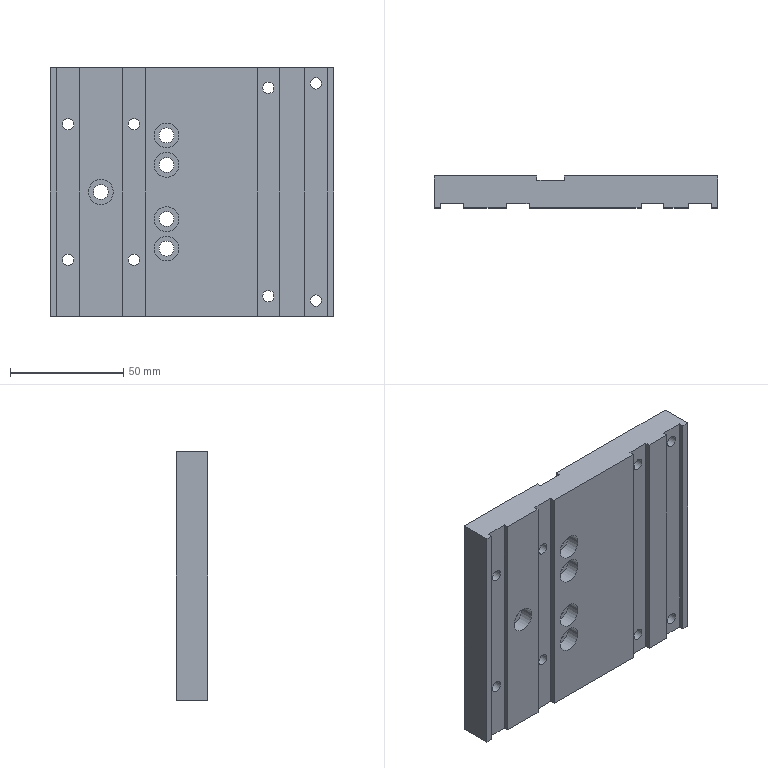Part | 1 solid | 49 faces | box 125.5 x 14 x 110 mm | volume 175999 mm3 | plane 31 | cylinder 18 | commonest cylinder face diameters 5 x8 6.6 x5 11 x5
STEP:
#1=CARTESIAN_POINT('',(93.5,0.,-78.5));
#2=VERTEX_POINT('',#1);
#3=CARTESIAN_POINT('',(93.5,0.,-76.));
#4=DIRECTION('',(0.,1.,0.));
#5=DIRECTION('',(0.,0.,-1.));
#6=AXIS2_PLACEMENT_3D('',#3,#4,#5);
#7=CIRCLE('',#6,2.5);
#8=EDGE_CURVE('',#2,#2,#7,.T.);
#9=ORIENTED_EDGE('',*,*,#8,.F.);
#10=EDGE_LOOP('',(#9));
#11=FACE_BOUND('',#10,.T.);
#12=CARTESIAN_POINT('',(93.5,12.,-78.5));
#13=VERTEX_POINT('',#12);
#14=CARTESIAN_POINT('',(93.5,12.,-76.));
#15=DIRECTION('',(0.,1.,0.));
#16=DIRECTION('',(0.,0.,-1.));
#17=AXIS2_PLACEMENT_3D('',#14,#15,#16);
#18=CIRCLE('',#17,2.5);
#19=EDGE_CURVE('',#13,#13,#18,.T.);
#20=ORIENTED_EDGE('',*,*,#19,.T.);
#21=EDGE_LOOP('',(#20));
#22=FACE_BOUND('',#21,.T.);
#23=CARTESIAN_POINT('',(93.5,12.001,-76.));
#24=DIRECTION('',(0.,-1.,0.));
#25=DIRECTION('',(0.,0.,1.));
#26=AXIS2_PLACEMENT_3D('',#23,#24,#25);
#27=CYLINDRICAL_SURFACE('',#26,2.5);
#28=ADVANCED_FACE('',(#11,#22),#27,.F.);
#29=CARTESIAN_POINT('',(93.5,0.,13.5));
#30=VERTEX_POINT('',#29);
#31=CARTESIAN_POINT('',(93.5,0.,16.));
#32=DIRECTION('',(0.,1.,0.));
#33=DIRECTION('',(0.,0.,-1.));
#34=AXIS2_PLACEMENT_3D('',#31,#32,#33);
#35=CIRCLE('',#34,2.5);
#36=EDGE_CURVE('',#30,#30,#35,.T.);
#37=ORIENTED_EDGE('',*,*,#36,.F.);
#38=EDGE_LOOP('',(#37));
#39=FACE_BOUND('',#38,.T.);
#40=CARTESIAN_POINT('',(93.5,12.,13.5));
#41=VERTEX_POINT('',#40);
#42=CARTESIAN_POINT('',(93.5,12.,16.));
#43=DIRECTION('',(0.,1.,0.));
#44=DIRECTION('',(0.,0.,-1.));
#45=AXIS2_PLACEMENT_3D('',#42,#43,#44);
#46=CIRCLE('',#45,2.5);
#47=EDGE_CURVE('',#41,#41,#46,.T.);
#48=ORIENTED_EDGE('',*,*,#47,.T.);
#49=EDGE_LOOP('',(#48));
#50=FACE_BOUND('',#49,.T.);
#51=CARTESIAN_POINT('',(93.5,12.001,16.));
#52=DIRECTION('',(0.,-1.,0.));
#53=DIRECTION('',(0.,0.,1.));
#54=AXIS2_PLACEMENT_3D('',#51,#52,#53);
#55=CYLINDRICAL_SURFACE('',#54,2.5);
#56=ADVANCED_FACE('',(#39,#50),#55,.F.);
#57=CARTESIAN_POINT('',(114.5,0.,-80.5));
#58=VERTEX_POINT('',#57);
#59=CARTESIAN_POINT('',(114.5,0.,-78.));
#60=DIRECTION('',(0.,-1.,0.));
#61=DIRECTION('',(0.,0.,-1.));
#62=AXIS2_PLACEMENT_3D('',#59,#60,#61);
#63=CIRCLE('',#62,2.5);
#64=EDGE_CURVE('',#58,#58,#63,.T.);
#65=ORIENTED_EDGE('',*,*,#64,.T.);
#66=EDGE_LOOP('',(#65));
#67=FACE_BOUND('',#66,.T.);
#68=CARTESIAN_POINT('',(114.5,12.,-80.5));
#69=VERTEX_POINT('',#68);
#70=CARTESIAN_POINT('',(114.5,12.,-78.));
#71=DIRECTION('',(0.,1.,0.));
#72=DIRECTION('',(0.,0.,-1.));
#73=AXIS2_PLACEMENT_3D('',#70,#71,#72);
#74=CIRCLE('',#73,2.5);
#75=EDGE_CURVE('',#69,#69,#74,.T.);
#76=ORIENTED_EDGE('',*,*,#75,.T.);
#77=EDGE_LOOP('',(#76));
#78=FACE_BOUND('',#77,.T.);
#79=CARTESIAN_POINT('',(114.5,19.071,-78.));
#80=DIRECTION('',(0.,-1.,0.));
#81=DIRECTION('',(0.,0.,1.));
#82=AXIS2_PLACEMENT_3D('',#79,#80,#81);
#83=CYLINDRICAL_SURFACE('',#82,2.5);
#84=ADVANCED_FACE('',(#67,#78),#83,.F.);
#85=CARTESIAN_POINT('',(114.5,0.,15.5));
#86=VERTEX_POINT('',#85);
#87=CARTESIAN_POINT('',(114.5,0.,18.));
#88=DIRECTION('',(0.,-1.,0.));
#89=DIRECTION('',(0.,0.,-1.));
#90=AXIS2_PLACEMENT_3D('',#87,#88,#89);
#91=CIRCLE('',#90,2.5);
#92=EDGE_CURVE('',#86,#86,#91,.T.);
#93=ORIENTED_EDGE('',*,*,#92,.T.);
#94=EDGE_LOOP('',(#93));
#95=FACE_BOUND('',#94,.T.);
#96=CARTESIAN_POINT('',(114.5,12.,15.5));
#97=VERTEX_POINT('',#96);
#98=CARTESIAN_POINT('',(114.5,12.,18.));
#99=DIRECTION('',(0.,1.,0.));
#100=DIRECTION('',(0.,0.,-1.));
#101=AXIS2_PLACEMENT_3D('',#98,#99,#100);
#102=CIRCLE('',#101,2.5);
#103=EDGE_CURVE('',#97,#97,#102,.T.);
#104=ORIENTED_EDGE('',*,*,#103,.T.);
#105=EDGE_LOOP('',(#104));
#106=FACE_BOUND('',#105,.T.);
#107=CARTESIAN_POINT('',(114.5,19.071,18.));
#108=DIRECTION('',(0.,-1.,0.));
#109=DIRECTION('',(0.,0.,1.));
#110=AXIS2_PLACEMENT_3D('',#107,#108,#109);
#111=CYLINDRICAL_SURFACE('',#110,2.5);
#112=ADVANCED_FACE('',(#95,#106),#111,.F.);
#113=CARTESIAN_POINT('',(34.,0.,-62.5));
#114=VERTEX_POINT('',#113);
#115=CARTESIAN_POINT('',(34.,0.,-60.));
#116=DIRECTION('',(0.,-1.,0.));
#117=DIRECTION('',(0.,0.,-1.));
#118=AXIS2_PLACEMENT_3D('',#115,#116,#117);
#119=CIRCLE('',#118,2.5);
#120=EDGE_CURVE('',#114,#114,#119,.T.);
#121=ORIENTED_EDGE('',*,*,#120,.T.);
#122=EDGE_LOOP('',(#121));
#123=FACE_BOUND('',#122,.T.);
#124=CARTESIAN_POINT('',(34.,12.,-62.5));
#125=VERTEX_POINT('',#124);
#126=CARTESIAN_POINT('',(34.,12.,-60.));
#127=DIRECTION('',(0.,1.,0.));
#128=DIRECTION('',(0.,0.,-1.));
#129=AXIS2_PLACEMENT_3D('',#126,#127,#128);
#130=CIRCLE('',#129,2.5);
#131=EDGE_CURVE('',#125,#125,#130,.T.);
#132=ORIENTED_EDGE('',*,*,#131,.T.);
#133=EDGE_LOOP('',(#132));
#134=FACE_BOUND('',#133,.T.);
#135=CARTESIAN_POINT('',(34.,19.071,-60.));
#136=DIRECTION('',(0.,-1.,0.));
#137=DIRECTION('',(0.,0.,1.));
#138=AXIS2_PLACEMENT_3D('',#135,#136,#137);
#139=CYLINDRICAL_SURFACE('',#138,2.5);
#140=ADVANCED_FACE('',(#123,#134),#139,.F.);
#141=CARTESIAN_POINT('',(34.,0.,-2.5));
#142=VERTEX_POINT('',#141);
#143=CARTESIAN_POINT('',(34.,0.,0.));
#144=DIRECTION('',(0.,-1.,0.));
#145=DIRECTION('',(0.,0.,-1.));
#146=AXIS2_PLACEMENT_3D('',#143,#144,#145);
#147=CIRCLE('',#146,2.5);
#148=EDGE_CURVE('',#142,#142,#147,.T.);
#149=ORIENTED_EDGE('',*,*,#148,.T.);
#150=EDGE_LOOP('',(#149));
#151=FACE_BOUND('',#150,.T.);
#152=CARTESIAN_POINT('',(34.,12.,-2.5));
#153=VERTEX_POINT('',#152);
#154=CARTESIAN_POINT('',(34.,12.,0.));
#155=DIRECTION('',(0.,1.,0.));
#156=DIRECTION('',(0.,0.,-1.));
#157=AXIS2_PLACEMENT_3D('',#154,#155,#156);
#158=CIRCLE('',#157,2.5);
#159=EDGE_CURVE('',#153,#153,#158,.T.);
#160=ORIENTED_EDGE('',*,*,#159,.T.);
#161=EDGE_LOOP('',(#160));
#162=FACE_BOUND('',#161,.T.);
#163=CARTESIAN_POINT('',(34.,19.071,0.));
#164=DIRECTION('',(0.,-1.,0.));
#165=DIRECTION('',(0.,0.,1.));
#166=AXIS2_PLACEMENT_3D('',#163,#164,#165);
#167=CYLINDRICAL_SURFACE('',#166,2.5);
#168=ADVANCED_FACE('',(#151,#162),#167,.F.);
#169=CARTESIAN_POINT('',(5.,0.,-62.5));
#170=VERTEX_POINT('',#169);
#171=CARTESIAN_POINT('',(5.,0.,-60.));
#172=DIRECTION('',(0.,-1.,0.));
#173=DIRECTION('',(0.,0.,-1.));
#174=AXIS2_PLACEMENT_3D('',#171,#172,#173);
#175=CIRCLE('',#174,2.5);
#176=EDGE_CURVE('',#170,#170,#175,.T.);
#177=ORIENTED_EDGE('',*,*,#176,.T.);
#178=EDGE_LOOP('',(#177));
#179=FACE_BOUND('',#178,.T.);
#180=CARTESIAN_POINT('',(5.,12.,-62.5));
#181=VERTEX_POINT('',#180);
#182=CARTESIAN_POINT('',(5.,12.,-60.));
#183=DIRECTION('',(0.,1.,0.));
#184=DIRECTION('',(0.,0.,-1.));
#185=AXIS2_PLACEMENT_3D('',#182,#183,#184);
#186=CIRCLE('',#185,2.5);
#187=EDGE_CURVE('',#181,#181,#186,.T.);
#188=ORIENTED_EDGE('',*,*,#187,.T.);
#189=EDGE_LOOP('',(#188));
#190=FACE_BOUND('',#189,.T.);
#191=CARTESIAN_POINT('',(5.,19.071,-60.));
#192=DIRECTION('',(0.,-1.,0.));
#193=DIRECTION('',(0.,0.,1.));
#194=AXIS2_PLACEMENT_3D('',#191,#192,#193);
#195=CYLINDRICAL_SURFACE('',#194,2.5);
#196=ADVANCED_FACE('',(#179,#190),#195,.F.);
#197=CARTESIAN_POINT('',(5.,0.,-2.5));
#198=VERTEX_POINT('',#197);
#199=CARTESIAN_POINT('',(5.,0.,0.));
#200=DIRECTION('',(0.,-1.,0.));
#201=DIRECTION('',(0.,0.,-1.));
#202=AXIS2_PLACEMENT_3D('',#199,#200,#201);
#203=CIRCLE('',#202,2.5);
#204=EDGE_CURVE('',#198,#198,#203,.T.);
#205=ORIENTED_EDGE('',*,*,#204,.T.);
#206=EDGE_LOOP('',(#205));
#207=FACE_BOUND('',#206,.T.);
#208=CARTESIAN_POINT('',(5.,12.,-2.5));
#209=VERTEX_POINT('',#208);
#210=CARTESIAN_POINT('',(5.,12.,0.));
#211=DIRECTION('',(0.,1.,0.));
#212=DIRECTION('',(0.,0.,-1.));
#213=AXIS2_PLACEMENT_3D('',#210,#211,#212);
#214=CIRCLE('',#213,2.5);
#215=EDGE_CURVE('',#209,#209,#214,.T.);
#216=ORIENTED_EDGE('',*,*,#215,.T.);
#217=EDGE_LOOP('',(#216));
#218=FACE_BOUND('',#217,.T.);
#219=CARTESIAN_POINT('',(5.,19.071,0.));
#220=DIRECTION('',(0.,-1.,0.));
#221=DIRECTION('',(0.,0.,1.));
#222=AXIS2_PLACEMENT_3D('',#219,#220,#221);
#223=CYLINDRICAL_SURFACE('',#222,2.5);
#224=ADVANCED_FACE('',(#207,#218),#223,.F.);
#225=CARTESIAN_POINT('',(19.5,-2.,-35.5));
#226=VERTEX_POINT('',#225);
#227=CARTESIAN_POINT('',(19.5,-2.,-30.));
#228=DIRECTION('',(0.,-1.,0.));
#229=DIRECTION('',(0.,0.,-1.));
#230=AXIS2_PLACEMENT_3D('',#227,#228,#229);
#231=CIRCLE('',#230,5.5);
#232=EDGE_CURVE('',#226,#226,#231,.T.);
#233=ORIENTED_EDGE('',*,*,#232,.T.);
#234=EDGE_LOOP('',(#233));
#235=FACE_BOUND('',#234,.T.);
#236=CARTESIAN_POINT('',(19.5,4.,-35.5));
#237=VERTEX_POINT('',#236);
#238=CARTESIAN_POINT('',(19.5,4.,-30.));
#239=DIRECTION('',(0.,-1.,0.));
#240=DIRECTION('',(0.,0.,-1.));
#241=AXIS2_PLACEMENT_3D('',#238,#239,#240);
#242=CIRCLE('',#241,5.5);
#243=EDGE_CURVE('',#237,#237,#242,.T.);
#244=ORIENTED_EDGE('',*,*,#243,.F.);
#245=EDGE_LOOP('',(#244));
#246=FACE_BOUND('',#245,.T.);
#247=CARTESIAN_POINT('',(19.5,4.,-30.));
#248=DIRECTION('',(0.,-1.,0.));
#249=DIRECTION('',(0.,0.,1.));
#250=AXIS2_PLACEMENT_3D('',#247,#248,#249);
#251=CYLINDRICAL_SURFACE('',#250,5.5);
#252=ADVANCED_FACE('',(#235,#246),#251,.F.);
#253=CARTESIAN_POINT('',(48.5,-2.,-60.5));
#254=VERTEX_POINT('',#253);
#255=CARTESIAN_POINT('',(48.5,-2.,-55.));
#256=DIRECTION('',(0.,-1.,0.));
#257=DIRECTION('',(0.,0.,-1.));
#258=AXIS2_PLACEMENT_3D('',#255,#256,#257);
#259=CIRCLE('',#258,5.5);
#260=EDGE_CURVE('',#254,#254,#259,.T.);
#261=ORIENTED_EDGE('',*,*,#260,.T.);
#262=EDGE_LOOP('',(#261));
#263=FACE_BOUND('',#262,.T.);
#264=CARTESIAN_POINT('',(48.5,4.,-60.5));
#265=VERTEX_POINT('',#264);
#266=CARTESIAN_POINT('',(48.5,4.,-55.));
#267=DIRECTION('',(0.,-1.,0.));
#268=DIRECTION('',(0.,0.,-1.));
#269=AXIS2_PLACEMENT_3D('',#266,#267,#268);
#270=CIRCLE('',#269,5.5);
#271=EDGE_CURVE('',#265,#265,#270,.T.);
#272=ORIENTED_EDGE('',*,*,#271,.F.);
#273=EDGE_LOOP('',(#272));
#274=FACE_BOUND('',#273,.T.);
#275=CARTESIAN_POINT('',(48.5,4.,-55.));
#276=DIRECTION('',(0.,-1.,0.));
#277=DIRECTION('',(0.,0.,1.));
#278=AXIS2_PLACEMENT_3D('',#275,#276,#277);
#279=CYLINDRICAL_SURFACE('',#278,5.5);
#280=ADVANCED_FACE('',(#263,#274),#279,.F.);
#281=CARTESIAN_POINT('',(48.5,-2.,-47.5));
#282=VERTEX_POINT('',#281);
#283=CARTESIAN_POINT('',(48.5,-2.,-42.));
#284=DIRECTION('',(0.,-1.,0.));
#285=DIRECTION('',(0.,0.,-1.));
#286=AXIS2_PLACEMENT_3D('',#283,#284,#285);
#287=CIRCLE('',#286,5.5);
#288=EDGE_CURVE('',#282,#282,#287,.T.);
#289=ORIENTED_EDGE('',*,*,#288,.T.);
#290=EDGE_LOOP('',(#289));
#291=FACE_BOUND('',#290,.T.);
#292=CARTESIAN_POINT('',(48.5,4.,-47.5));
#293=VERTEX_POINT('',#292);
#294=CARTESIAN_POINT('',(48.5,4.,-42.));
#295=DIRECTION('',(0.,-1.,0.));
#296=DIRECTION('',(0.,0.,-1.));
#297=AXIS2_PLACEMENT_3D('',#294,#295,#296);
#298=CIRCLE('',#297,5.5);
#299=EDGE_CURVE('',#293,#293,#298,.T.);
#300=ORIENTED_EDGE('',*,*,#299,.F.);
#301=EDGE_LOOP('',(#300));
#302=FACE_BOUND('',#301,.T.);
#303=CARTESIAN_POINT('',(48.5,4.,-42.));
#304=DIRECTION('',(0.,-1.,0.));
#305=DIRECTION('',(0.,0.,1.));
#306=AXIS2_PLACEMENT_3D('',#303,#304,#305);
#307=CYLINDRICAL_SURFACE('',#306,5.5);
#308=ADVANCED_FACE('',(#291,#302),#307,.F.);
#309=CARTESIAN_POINT('',(48.5,-2.,-10.5));
#310=VERTEX_POINT('',#309);
#311=CARTESIAN_POINT('',(48.5,-2.,-5.));
#312=DIRECTION('',(0.,-1.,0.));
#313=DIRECTION('',(0.,0.,-1.));
#314=AXIS2_PLACEMENT_3D('',#311,#312,#313);
#315=CIRCLE('',#314,5.5);
#316=EDGE_CURVE('',#310,#310,#315,.T.);
#317=ORIENTED_EDGE('',*,*,#316,.T.);
#318=EDGE_LOOP('',(#317));
#319=FACE_BOUND('',#318,.T.);
#320=CARTESIAN_POINT('',(48.5,4.,-10.5));
#321=VERTEX_POINT('',#320);
#322=CARTESIAN_POINT('',(48.5,4.,-5.));
#323=DIRECTION('',(0.,-1.,0.));
#324=DIRECTION('',(0.,0.,-1.));
#325=AXIS2_PLACEMENT_3D('',#322,#323,#324);
#326=CIRCLE('',#325,5.5);
#327=EDGE_CURVE('',#321,#321,#326,.T.);
#328=ORIENTED_EDGE('',*,*,#327,.F.);
#329=EDGE_LOOP('',(#328));
#330=FACE_BOUND('',#329,.T.);
#331=CARTESIAN_POINT('',(48.5,4.,-5.));
#332=DIRECTION('',(0.,-1.,0.));
#333=DIRECTION('',(0.,0.,1.));
#334=AXIS2_PLACEMENT_3D('',#331,#332,#333);
#335=CYLINDRICAL_SURFACE('',#334,5.5);
#336=ADVANCED_FACE('',(#319,#330),#335,.F.);
#337=CARTESIAN_POINT('',(48.5,-2.,-23.5));
#338=VERTEX_POINT('',#337);
#339=CARTESIAN_POINT('',(48.5,-2.,-18.));
#340=DIRECTION('',(0.,-1.,0.));
#341=DIRECTION('',(0.,0.,-1.));
#342=AXIS2_PLACEMENT_3D('',#339,#340,#341);
#343=CIRCLE('',#342,5.5);
#344=EDGE_CURVE('',#338,#338,#343,.T.);
#345=ORIENTED_EDGE('',*,*,#344,.T.);
#346=EDGE_LOOP('',(#345));
#347=FACE_BOUND('',#346,.T.);
#348=CARTESIAN_POINT('',(48.5,4.,-23.5));
#349=VERTEX_POINT('',#348);
#350=CARTESIAN_POINT('',(48.5,4.,-18.));
#351=DIRECTION('',(0.,-1.,0.));
#352=DIRECTION('',(0.,0.,-1.));
#353=AXIS2_PLACEMENT_3D('',#350,#351,#352);
#354=CIRCLE('',#353,5.5);
#355=EDGE_CURVE('',#349,#349,#354,.T.);
#356=ORIENTED_EDGE('',*,*,#355,.F.);
#357=EDGE_LOOP('',(#356));
#358=FACE_BOUND('',#357,.T.);
#359=CARTESIAN_POINT('',(48.5,4.,-18.));
#360=DIRECTION('',(0.,-1.,0.));
#361=DIRECTION('',(0.,0.,1.));
#362=AXIS2_PLACEMENT_3D('',#359,#360,#361);
#363=CYLINDRICAL_SURFACE('',#362,5.5);
#364=ADVANCED_FACE('',(#347,#358),#363,.F.);
#365=CARTESIAN_POINT('',(48.5,4.,-21.3));
#366=VERTEX_POINT('',#365);
#367=CARTESIAN_POINT('',(48.5,4.,-18.));
#368=DIRECTION('',(0.,1.,0.));
#369=DIRECTION('',(0.,0.,-1.));
#370=AXIS2_PLACEMENT_3D('',#367,#368,#369);
#371=CIRCLE('',#370,3.3);
#372=EDGE_CURVE('',#366,#366,#371,.T.);
#373=ORIENTED_EDGE('',*,*,#372,.F.);
#374=EDGE_LOOP('',(#373));
#375=FACE_BOUND('',#374,.T.);
#376=CARTESIAN_POINT('',(48.5,10.,-21.3));
#377=VERTEX_POINT('',#376);
#378=CARTESIAN_POINT('',(48.5,10.,-18.));
#379=DIRECTION('',(0.,1.,0.));
#380=DIRECTION('',(0.,0.,-1.));
#381=AXIS2_PLACEMENT_3D('',#378,#379,#380);
#382=CIRCLE('',#381,3.3);
#383=EDGE_CURVE('',#377,#377,#382,.T.);
#384=ORIENTED_EDGE('',*,*,#383,.T.);
#385=EDGE_LOOP('',(#384));
#386=FACE_BOUND('',#385,.T.);
#387=CARTESIAN_POINT('',(48.5,12.001,-18.));
#388=DIRECTION('',(0.,-1.,0.));
#389=DIRECTION('',(0.,0.,1.));
#390=AXIS2_PLACEMENT_3D('',#387,#388,#389);
#391=CYLINDRICAL_SURFACE('',#390,3.3);
#392=ADVANCED_FACE('',(#375,#386),#391,.F.);
#393=CARTESIAN_POINT('',(48.5,4.,-8.3));
#394=VERTEX_POINT('',#393);
#395=CARTESIAN_POINT('',(48.5,4.,-5.));
#396=DIRECTION('',(0.,1.,0.));
#397=DIRECTION('',(0.,0.,-1.));
#398=AXIS2_PLACEMENT_3D('',#395,#396,#397);
#399=CIRCLE('',#398,3.3);
#400=EDGE_CURVE('',#394,#394,#399,.T.);
#401=ORIENTED_EDGE('',*,*,#400,.F.);
#402=EDGE_LOOP('',(#401));
#403=FACE_BOUND('',#402,.T.);
#404=CARTESIAN_POINT('',(48.5,10.,-8.3));
#405=VERTEX_POINT('',#404);
#406=CARTESIAN_POINT('',(48.5,10.,-5.));
#407=DIRECTION('',(0.,1.,0.));
#408=DIRECTION('',(0.,0.,-1.));
#409=AXIS2_PLACEMENT_3D('',#406,#407,#408);
#410=CIRCLE('',#409,3.3);
#411=EDGE_CURVE('',#405,#405,#410,.T.);
#412=ORIENTED_EDGE('',*,*,#411,.T.);
#413=EDGE_LOOP('',(#412));
#414=FACE_BOUND('',#413,.T.);
#415=CARTESIAN_POINT('',(48.5,12.001,-5.));
#416=DIRECTION('',(0.,-1.,0.));
#417=DIRECTION('',(0.,0.,1.));
#418=AXIS2_PLACEMENT_3D('',#415,#416,#417);
#419=CYLINDRICAL_SURFACE('',#418,3.3);
#420=ADVANCED_FACE('',(#403,#414),#419,.F.);
#421=CARTESIAN_POINT('',(48.5,4.,-45.3));
#422=VERTEX_POINT('',#421);
#423=CARTESIAN_POINT('',(48.5,4.,-42.));
#424=DIRECTION('',(0.,1.,0.));
#425=DIRECTION('',(0.,0.,-1.));
#426=AXIS2_PLACEMENT_3D('',#423,#424,#425);
#427=CIRCLE('',#426,3.3);
#428=EDGE_CURVE('',#422,#422,#427,.T.);
#429=ORIENTED_EDGE('',*,*,#428,.F.);
#430=EDGE_LOOP('',(#429));
#431=FACE_BOUND('',#430,.T.);
#432=CARTESIAN_POINT('',(48.5,10.,-45.3));
#433=VERTEX_POINT('',#432);
#434=CARTESIAN_POINT('',(48.5,10.,-42.));
#435=DIRECTION('',(0.,1.,0.));
#436=DIRECTION('',(0.,0.,-1.));
#437=AXIS2_PLACEMENT_3D('',#434,#435,#436);
#438=CIRCLE('',#437,3.3);
#439=EDGE_CURVE('',#433,#433,#438,.T.);
#440=ORIENTED_EDGE('',*,*,#439,.T.);
#441=EDGE_LOOP('',(#440));
#442=FACE_BOUND('',#441,.T.);
#443=CARTESIAN_POINT('',(48.5,12.001,-42.));
#444=DIRECTION('',(0.,-1.,0.));
#445=DIRECTION('',(0.,0.,1.));
#446=AXIS2_PLACEMENT_3D('',#443,#444,#445);
#447=CYLINDRICAL_SURFACE('',#446,3.3);
#448=ADVANCED_FACE('',(#431,#442),#447,.F.);
#449=CARTESIAN_POINT('',(48.5,4.,-58.3));
#450=VERTEX_POINT('',#449);
#451=CARTESIAN_POINT('',(48.5,4.,-55.));
#452=DIRECTION('',(0.,1.,0.));
#453=DIRECTION('',(0.,0.,-1.));
#454=AXIS2_PLACEMENT_3D('',#451,#452,#453);
#455=CIRCLE('',#454,3.3);
#456=EDGE_CURVE('',#450,#450,#455,.T.);
#457=ORIENTED_EDGE('',*,*,#456,.F.);
#458=EDGE_LOOP('',(#457));
#459=FACE_BOUND('',#458,.T.);
#460=CARTESIAN_POINT('',(48.5,10.,-58.3));
#461=VERTEX_POINT('',#460);
#462=CARTESIAN_POINT('',(48.5,10.,-55.));
#463=DIRECTION('',(0.,1.,0.));
#464=DIRECTION('',(0.,0.,-1.));
#465=AXIS2_PLACEMENT_3D('',#462,#463,#464);
#466=CIRCLE('',#465,3.3);
#467=EDGE_CURVE('',#461,#461,#466,.T.);
#468=ORIENTED_EDGE('',*,*,#467,.T.);
#469=EDGE_LOOP('',(#468));
#470=FACE_BOUND('',#469,.T.);
#471=CARTESIAN_POINT('',(48.5,12.001,-55.));
#472=DIRECTION('',(0.,-1.,0.));
#473=DIRECTION('',(0.,0.,1.));
#474=AXIS2_PLACEMENT_3D('',#471,#472,#473);
#475=CYLINDRICAL_SURFACE('',#474,3.3);
#476=ADVANCED_FACE('',(#459,#470),#475,.F.);
#477=CARTESIAN_POINT('',(19.5,4.,-33.3));
#478=VERTEX_POINT('',#477);
#479=CARTESIAN_POINT('',(19.5,4.,-30.));
#480=DIRECTION('',(0.,1.,0.));
#481=DIRECTION('',(0.,0.,-1.));
#482=AXIS2_PLACEMENT_3D('',#479,#480,#481);
#483=CIRCLE('',#482,3.3);
#484=EDGE_CURVE('',#478,#478,#483,.T.);
#485=ORIENTED_EDGE('',*,*,#484,.F.);
#486=EDGE_LOOP('',(#485));
#487=FACE_BOUND('',#486,.T.);
#488=CARTESIAN_POINT('',(19.5,12.,-33.3));
#489=VERTEX_POINT('',#488);
#490=CARTESIAN_POINT('',(19.5,12.,-30.));
#491=DIRECTION('',(0.,1.,0.));
#492=DIRECTION('',(0.,0.,-1.));
#493=AXIS2_PLACEMENT_3D('',#490,#491,#492);
#494=CIRCLE('',#493,3.3);
#495=EDGE_CURVE('',#489,#489,#494,.T.);
#496=ORIENTED_EDGE('',*,*,#495,.T.);
#497=EDGE_LOOP('',(#496));
#498=FACE_BOUND('',#497,.T.);
#499=CARTESIAN_POINT('',(19.5,12.001,-30.));
#500=DIRECTION('',(0.,-1.,0.));
#501=DIRECTION('',(0.,0.,1.));
#502=AXIS2_PLACEMENT_3D('',#499,#500,#501);
#503=CYLINDRICAL_SURFACE('',#502,3.3);
#504=ADVANCED_FACE('',(#487,#498),#503,.F.);
#505=CARTESIAN_POINT('',(88.5,-2.,25.));
#506=VERTEX_POINT('',#505);
#507=CARTESIAN_POINT('',(88.5,-2.,-85.));
#508=VERTEX_POINT('',#507);
#509=CARTESIAN_POINT('',(88.5,-2.,-85.));
#510=DIRECTION('',(0.,0.,-1.));
#511=VECTOR('',#510,1000.);
#512=LINE('',#509,#511);
#513=EDGE_CURVE('',#506,#508,#512,.T.);
#514=ORIENTED_EDGE('',*,*,#513,.F.);
#515=CARTESIAN_POINT('',(39.,-2.,25.));
#516=VERTEX_POINT('',#515);
#517=CARTESIAN_POINT('',(-3.,-2.,25.));
#518=DIRECTION('',(-1.,0.,0.));
#519=VECTOR('',#518,1000.);
#520=LINE('',#517,#519);
#521=EDGE_CURVE('',#506,#516,#520,.T.);
#522=ORIENTED_EDGE('',*,*,#521,.T.);
#523=CARTESIAN_POINT('',(39.,-2.,-85.));
#524=VERTEX_POINT('',#523);
#525=CARTESIAN_POINT('',(39.,-2.,25.));
#526=DIRECTION('',(0.,0.,1.));
#527=VECTOR('',#526,1000.);
#528=LINE('',#525,#527);
#529=EDGE_CURVE('',#524,#516,#528,.T.);
#530=ORIENTED_EDGE('',*,*,#529,.F.);
#531=CARTESIAN_POINT('',(-3.,-2.,-85.));
#532=DIRECTION('',(1.,0.,0.));
#533=VECTOR('',#532,1000.);
#534=LINE('',#531,#533);
#535=EDGE_CURVE('',#524,#508,#534,.T.);
#536=ORIENTED_EDGE('',*,*,#535,.T.);
#537=EDGE_LOOP('',(#514,#522,#530,#536));
#538=FACE_BOUND('',#537,.T.);
#539=ORIENTED_EDGE('',*,*,#344,.F.);
#540=EDGE_LOOP('',(#539));
#541=FACE_BOUND('',#540,.T.);
#542=ORIENTED_EDGE('',*,*,#316,.F.);
#543=EDGE_LOOP('',(#542));
#544=FACE_BOUND('',#543,.T.);
#545=ORIENTED_EDGE('',*,*,#288,.F.);
#546=EDGE_LOOP('',(#545));
#547=FACE_BOUND('',#546,.T.);
#548=ORIENTED_EDGE('',*,*,#260,.F.);
#549=EDGE_LOOP('',(#548));
#550=FACE_BOUND('',#549,.T.);
#551=CARTESIAN_POINT('',(0.,-2.,0.));
#552=DIRECTION('',(0.,-1.,0.));
#553=DIRECTION('',(0.,0.,1.));
#554=AXIS2_PLACEMENT_3D('',#551,#552,#553);
#555=PLANE('',#554);
#556=ADVANCED_FACE('',(#538,#541,#544,#547,#550),#555,.T.);
#557=ORIENTED_EDGE('',*,*,#19,.F.);
#558=EDGE_LOOP('',(#557));
#559=FACE_BOUND('',#558,.T.);
#560=ORIENTED_EDGE('',*,*,#47,.F.);
#561=EDGE_LOOP('',(#560));
#562=FACE_BOUND('',#561,.T.);
#563=ORIENTED_EDGE('',*,*,#75,.F.);
#564=EDGE_LOOP('',(#563));
#565=FACE_BOUND('',#564,.T.);
#566=ORIENTED_EDGE('',*,*,#103,.F.);
#567=EDGE_LOOP('',(#566));
#568=FACE_BOUND('',#567,.T.);
#569=CARTESIAN_POINT('',(122.5,12.,-85.));
#570=VERTEX_POINT('',#569);
#571=CARTESIAN_POINT('',(54.5,12.,-85.));
#572=VERTEX_POINT('',#571);
#573=CARTESIAN_POINT('',(0.,12.,-85.));
#574=DIRECTION('',(-1.,0.,0.));
#575=VECTOR('',#574,1000.);
#576=LINE('',#573,#575);
#577=EDGE_CURVE('',#570,#572,#576,.T.);
#578=ORIENTED_EDGE('',*,*,#577,.T.);
#579=CARTESIAN_POINT('',(54.5,12.,25.));
#580=VERTEX_POINT('',#579);
#581=CARTESIAN_POINT('',(54.5,12.,25.));
#582=DIRECTION('',(0.,0.,-1.));
#583=VECTOR('',#582,1000.);
#584=LINE('',#581,#583);
#585=EDGE_CURVE('',#580,#572,#584,.T.);
#586=ORIENTED_EDGE('',*,*,#585,.F.);
#587=CARTESIAN_POINT('',(122.5,12.,25.));
#588=VERTEX_POINT('',#587);
#589=CARTESIAN_POINT('',(0.,12.,25.));
#590=DIRECTION('',(1.,0.,0.));
#591=VECTOR('',#590,1000.);
#592=LINE('',#589,#591);
#593=EDGE_CURVE('',#580,#588,#592,.T.);
#594=ORIENTED_EDGE('',*,*,#593,.T.);
#595=CARTESIAN_POINT('',(122.5,12.,0.));
#596=DIRECTION('',(0.,0.,-1.));
#597=VECTOR('',#596,1000.);
#598=LINE('',#595,#597);
#599=EDGE_CURVE('',#588,#570,#598,.T.);
#600=ORIENTED_EDGE('',*,*,#599,.T.);
#601=EDGE_LOOP('',(#578,#586,#594,#600));
#602=FACE_BOUND('',#601,.T.);
#603=CARTESIAN_POINT('',(0.,12.,0.));
#604=DIRECTION('',(0.,-1.,0.));
#605=DIRECTION('',(0.,0.,1.));
#606=AXIS2_PLACEMENT_3D('',#603,#604,#605);
#607=PLANE('',#606);
#608=ADVANCED_FACE('',(#559,#562,#565,#568,#602),#607,.F.);
#609=CARTESIAN_POINT('',(98.5,-2.,-85.));
#610=VERTEX_POINT('',#609);
#611=CARTESIAN_POINT('',(98.5,-2.,25.));
#612=VERTEX_POINT('',#611);
#613=CARTESIAN_POINT('',(98.5,-2.,-85.));
#614=DIRECTION('',(0.,0.,1.));
#615=VECTOR('',#614,1000.);
#616=LINE('',#613,#615);
#617=EDGE_CURVE('',#610,#612,#616,.T.);
#618=ORIENTED_EDGE('',*,*,#617,.F.);
#619=CARTESIAN_POINT('',(109.5,-2.,-85.));
#620=VERTEX_POINT('',#619);
#621=CARTESIAN_POINT('',(-3.,-2.,-85.));
#622=DIRECTION('',(1.,0.,0.));
#623=VECTOR('',#622,1000.);
#624=LINE('',#621,#623);
#625=EDGE_CURVE('',#610,#620,#624,.T.);
#626=ORIENTED_EDGE('',*,*,#625,.T.);
#627=CARTESIAN_POINT('',(109.5,-2.,25.));
#628=VERTEX_POINT('',#627);
#629=CARTESIAN_POINT('',(109.5,-2.,25.));
#630=DIRECTION('',(0.,0.,-1.));
#631=VECTOR('',#630,1000.);
#632=LINE('',#629,#631);
#633=EDGE_CURVE('',#628,#620,#632,.T.);
#634=ORIENTED_EDGE('',*,*,#633,.F.);
#635=CARTESIAN_POINT('',(-3.,-2.,25.));
#636=DIRECTION('',(-1.,0.,0.));
#637=VECTOR('',#636,1000.);
#638=LINE('',#635,#637);
#639=EDGE_CURVE('',#628,#612,#638,.T.);
#640=ORIENTED_EDGE('',*,*,#639,.T.);
#641=EDGE_LOOP('',(#618,#626,#634,#640));
#642=FACE_BOUND('',#641,.T.);
#643=CARTESIAN_POINT('',(0.,-2.,0.));
#644=DIRECTION('',(0.,-1.,0.));
#645=DIRECTION('',(0.,0.,1.));
#646=AXIS2_PLACEMENT_3D('',#643,#644,#645);
#647=PLANE('',#646);
#648=ADVANCED_FACE('',(#642),#647,.T.);
#649=ORIENTED_EDGE('',*,*,#232,.F.);
#650=EDGE_LOOP('',(#649));
#651=FACE_BOUND('',#650,.T.);
#652=CARTESIAN_POINT('',(29.,-2.,25.));
#653=VERTEX_POINT('',#652);
#654=CARTESIAN_POINT('',(29.,-2.,-85.));
#655=VERTEX_POINT('',#654);
#656=CARTESIAN_POINT('',(29.,-2.,25.));
#657=DIRECTION('',(0.,0.,-1.));
#658=VECTOR('',#657,1000.);
#659=LINE('',#656,#658);
#660=EDGE_CURVE('',#653,#655,#659,.T.);
#661=ORIENTED_EDGE('',*,*,#660,.F.);
#662=CARTESIAN_POINT('',(10.,-2.,25.));
#663=VERTEX_POINT('',#662);
#664=CARTESIAN_POINT('',(-3.,-2.,25.));
#665=DIRECTION('',(-1.,0.,0.));
#666=VECTOR('',#665,1000.);
#667=LINE('',#664,#666);
#668=EDGE_CURVE('',#653,#663,#667,.T.);
#669=ORIENTED_EDGE('',*,*,#668,.T.);
#670=CARTESIAN_POINT('',(10.,-2.,-85.));
#671=VERTEX_POINT('',#670);
#672=CARTESIAN_POINT('',(10.,-2.,25.));
#673=DIRECTION('',(0.,0.,1.));
#674=VECTOR('',#673,1000.);
#675=LINE('',#672,#674);
#676=EDGE_CURVE('',#671,#663,#675,.T.);
#677=ORIENTED_EDGE('',*,*,#676,.F.);
#678=CARTESIAN_POINT('',(-3.,-2.,-85.));
#679=DIRECTION('',(1.,0.,0.));
#680=VECTOR('',#679,1000.);
#681=LINE('',#678,#680);
#682=EDGE_CURVE('',#671,#655,#681,.T.);
#683=ORIENTED_EDGE('',*,*,#682,.T.);
#684=EDGE_LOOP('',(#661,#669,#677,#683));
#685=FACE_BOUND('',#684,.T.);
#686=CARTESIAN_POINT('',(0.,-2.,0.));
#687=DIRECTION('',(0.,-1.,0.));
#688=DIRECTION('',(0.,0.,1.));
#689=AXIS2_PLACEMENT_3D('',#686,#687,#688);
#690=PLANE('',#689);
#691=ADVANCED_FACE('',(#651,#685),#690,.T.);
#692=CARTESIAN_POINT('',(0.,-2.,25.));
#693=VERTEX_POINT('',#692);
#694=CARTESIAN_POINT('',(0.,-2.,-85.));
#695=VERTEX_POINT('',#694);
#696=CARTESIAN_POINT('',(0.,-2.,25.));
#697=DIRECTION('',(0.,0.,-1.));
#698=VECTOR('',#697,1000.);
#699=LINE('',#696,#698);
#700=EDGE_CURVE('',#693,#695,#699,.T.);
#701=ORIENTED_EDGE('',*,*,#700,.F.);
#702=CARTESIAN_POINT('',(-3.,-2.,25.));
#703=VERTEX_POINT('',#702);
#704=CARTESIAN_POINT('',(-3.,-2.,25.));
#705=DIRECTION('',(-1.,0.,0.));
#706=VECTOR('',#705,1000.);
#707=LINE('',#704,#706);
#708=EDGE_CURVE('',#693,#703,#707,.T.);
#709=ORIENTED_EDGE('',*,*,#708,.T.);
#710=CARTESIAN_POINT('',(-3.,-2.,-85.));
#711=VERTEX_POINT('',#710);
#712=CARTESIAN_POINT('',(-3.,-2.,25.));
#713=DIRECTION('',(0.,0.,-1.));
#714=VECTOR('',#713,1000.);
#715=LINE('',#712,#714);
#716=EDGE_CURVE('',#703,#711,#715,.T.);
#717=ORIENTED_EDGE('',*,*,#716,.T.);
#718=CARTESIAN_POINT('',(-3.,-2.,-85.));
#719=DIRECTION('',(1.,0.,0.));
#720=VECTOR('',#719,1000.);
#721=LINE('',#718,#720);
#722=EDGE_CURVE('',#711,#695,#721,.T.);
#723=ORIENTED_EDGE('',*,*,#722,.T.);
#724=EDGE_LOOP('',(#701,#709,#717,#723));
#725=FACE_BOUND('',#724,.T.);
#726=CARTESIAN_POINT('',(0.,-2.,0.));
#727=DIRECTION('',(0.,-1.,0.));
#728=DIRECTION('',(0.,0.,1.));
#729=AXIS2_PLACEMENT_3D('',#726,#727,#728);
#730=PLANE('',#729);
#731=ADVANCED_FACE('',(#725),#730,.T.);
#732=CARTESIAN_POINT('',(-3.,12.,-85.));
#733=VERTEX_POINT('',#732);
#734=CARTESIAN_POINT('',(-3.,10.,-85.));
#735=DIRECTION('',(0.,-1.,0.));
#736=VECTOR('',#735,1000.);
#737=LINE('',#734,#736);
#738=EDGE_CURVE('',#733,#711,#737,.T.);
#739=ORIENTED_EDGE('',*,*,#738,.T.);
#740=ORIENTED_EDGE('',*,*,#716,.F.);
#741=CARTESIAN_POINT('',(-3.,12.,25.));
#742=VERTEX_POINT('',#741);
#743=CARTESIAN_POINT('',(-3.,10.,25.));
#744=DIRECTION('',(0.,-1.,0.));
#745=VECTOR('',#744,1000.);
#746=LINE('',#743,#745);
#747=EDGE_CURVE('',#742,#703,#746,.T.);
#748=ORIENTED_EDGE('',*,*,#747,.F.);
#749=CARTESIAN_POINT('',(-3.,12.,0.));
#750=DIRECTION('',(0.,0.,1.));
#751=VECTOR('',#750,1000.);
#752=LINE('',#749,#751);
#753=EDGE_CURVE('',#733,#742,#752,.T.);
#754=ORIENTED_EDGE('',*,*,#753,.F.);
#755=EDGE_LOOP('',(#739,#740,#748,#754));
#756=FACE_BOUND('',#755,.T.);
#757=CARTESIAN_POINT('',(-3.,10.,0.));
#758=DIRECTION('',(1.,0.,0.));
#759=DIRECTION('',(0.,0.,1.));
#760=AXIS2_PLACEMENT_3D('',#757,#758,#759);
#761=PLANE('',#760);
#762=ADVANCED_FACE('',(#756),#761,.F.);
#763=ORIENTED_EDGE('',*,*,#521,.F.);
#764=CARTESIAN_POINT('',(88.5,0.,25.));
#765=VERTEX_POINT('',#764);
#766=CARTESIAN_POINT('',(88.5,0.,25.));
#767=DIRECTION('',(0.,-1.,0.));
#768=VECTOR('',#767,1000.);
#769=LINE('',#766,#768);
#770=EDGE_CURVE('',#765,#506,#769,.T.);
#771=ORIENTED_EDGE('',*,*,#770,.F.);
#772=CARTESIAN_POINT('',(98.5,0.,25.));
#773=VERTEX_POINT('',#772);
#774=CARTESIAN_POINT('',(98.5,0.,25.));
#775=DIRECTION('',(-1.,0.,0.));
#776=VECTOR('',#775,1000.);
#777=LINE('',#774,#776);
#778=EDGE_CURVE('',#773,#765,#777,.T.);
#779=ORIENTED_EDGE('',*,*,#778,.F.);
#780=CARTESIAN_POINT('',(98.5,0.,25.));
#781=DIRECTION('',(0.,-1.,0.));
#782=VECTOR('',#781,1000.);
#783=LINE('',#780,#782);
#784=EDGE_CURVE('',#773,#612,#783,.T.);
#785=ORIENTED_EDGE('',*,*,#784,.T.);
#786=ORIENTED_EDGE('',*,*,#639,.F.);
#787=CARTESIAN_POINT('',(109.5,0.,25.));
#788=VERTEX_POINT('',#787);
#789=CARTESIAN_POINT('',(109.5,0.,25.));
#790=DIRECTION('',(0.,-1.,0.));
#791=VECTOR('',#790,1000.);
#792=LINE('',#789,#791);
#793=EDGE_CURVE('',#788,#628,#792,.T.);
#794=ORIENTED_EDGE('',*,*,#793,.F.);
#795=CARTESIAN_POINT('',(119.5,0.,25.));
#796=VERTEX_POINT('',#795);
#797=CARTESIAN_POINT('',(109.5,0.,25.));
#798=DIRECTION('',(-1.,0.,0.));
#799=VECTOR('',#798,1000.);
#800=LINE('',#797,#799);
#801=EDGE_CURVE('',#796,#788,#800,.T.);
#802=ORIENTED_EDGE('',*,*,#801,.F.);
#803=CARTESIAN_POINT('',(119.5,-2.,25.));
#804=VERTEX_POINT('',#803);
#805=CARTESIAN_POINT('',(119.5,0.,25.));
#806=DIRECTION('',(0.,-1.,0.));
#807=VECTOR('',#806,1000.);
#808=LINE('',#805,#807);
#809=EDGE_CURVE('',#796,#804,#808,.T.);
#810=ORIENTED_EDGE('',*,*,#809,.T.);
#811=CARTESIAN_POINT('',(122.5,-2.,25.));
#812=VERTEX_POINT('',#811);
#813=CARTESIAN_POINT('',(-3.,-2.,25.));
#814=DIRECTION('',(-1.,0.,0.));
#815=VECTOR('',#814,1000.);
#816=LINE('',#813,#815);
#817=EDGE_CURVE('',#812,#804,#816,.T.);
#818=ORIENTED_EDGE('',*,*,#817,.F.);
#819=CARTESIAN_POINT('',(122.5,10.,25.));
#820=DIRECTION('',(0.,-1.,0.));
#821=VECTOR('',#820,1000.);
#822=LINE('',#819,#821);
#823=EDGE_CURVE('',#588,#812,#822,.T.);
#824=ORIENTED_EDGE('',*,*,#823,.F.);
#825=ORIENTED_EDGE('',*,*,#593,.F.);
#826=CARTESIAN_POINT('',(54.5,10.,25.));
#827=VERTEX_POINT('',#826);
#828=CARTESIAN_POINT('',(54.5,10.,25.));
#829=DIRECTION('',(0.,1.,0.));
#830=VECTOR('',#829,1000.);
#831=LINE('',#828,#830);
#832=EDGE_CURVE('',#827,#580,#831,.T.);
#833=ORIENTED_EDGE('',*,*,#832,.F.);
#834=CARTESIAN_POINT('',(42.5,10.,25.));
#835=VERTEX_POINT('',#834);
#836=CARTESIAN_POINT('',(42.5,10.,25.));
#837=DIRECTION('',(1.,0.,0.));
#838=VECTOR('',#837,1000.);
#839=LINE('',#836,#838);
#840=EDGE_CURVE('',#835,#827,#839,.T.);
#841=ORIENTED_EDGE('',*,*,#840,.F.);
#842=CARTESIAN_POINT('',(42.5,12.,25.));
#843=VERTEX_POINT('',#842);
#844=CARTESIAN_POINT('',(42.5,10.,25.));
#845=DIRECTION('',(0.,1.,0.));
#846=VECTOR('',#845,1000.);
#847=LINE('',#844,#846);
#848=EDGE_CURVE('',#835,#843,#847,.T.);
#849=ORIENTED_EDGE('',*,*,#848,.T.);
#850=CARTESIAN_POINT('',(0.,12.,25.));
#851=DIRECTION('',(1.,0.,0.));
#852=VECTOR('',#851,1000.);
#853=LINE('',#850,#852);
#854=EDGE_CURVE('',#742,#843,#853,.T.);
#855=ORIENTED_EDGE('',*,*,#854,.F.);
#856=ORIENTED_EDGE('',*,*,#747,.T.);
#857=ORIENTED_EDGE('',*,*,#708,.F.);
#858=CARTESIAN_POINT('',(0.,0.,25.));
#859=VERTEX_POINT('',#858);
#860=CARTESIAN_POINT('',(0.,0.,25.));
#861=DIRECTION('',(0.,-1.,0.));
#862=VECTOR('',#861,1000.);
#863=LINE('',#860,#862);
#864=EDGE_CURVE('',#859,#693,#863,.T.);
#865=ORIENTED_EDGE('',*,*,#864,.F.);
#866=CARTESIAN_POINT('',(10.,0.,25.));
#867=VERTEX_POINT('',#866);
#868=CARTESIAN_POINT('',(0.,0.,25.));
#869=DIRECTION('',(-1.,0.,0.));
#870=VECTOR('',#869,1000.);
#871=LINE('',#868,#870);
#872=EDGE_CURVE('',#867,#859,#871,.T.);
#873=ORIENTED_EDGE('',*,*,#872,.F.);
#874=CARTESIAN_POINT('',(10.,0.,25.));
#875=DIRECTION('',(0.,-1.,0.));
#876=VECTOR('',#875,1000.);
#877=LINE('',#874,#876);
#878=EDGE_CURVE('',#867,#663,#877,.T.);
#879=ORIENTED_EDGE('',*,*,#878,.T.);
#880=ORIENTED_EDGE('',*,*,#668,.F.);
#881=CARTESIAN_POINT('',(29.,0.,25.));
#882=VERTEX_POINT('',#881);
#883=CARTESIAN_POINT('',(29.,0.,25.));
#884=DIRECTION('',(0.,-1.,0.));
#885=VECTOR('',#884,1000.);
#886=LINE('',#883,#885);
#887=EDGE_CURVE('',#882,#653,#886,.T.);
#888=ORIENTED_EDGE('',*,*,#887,.F.);
#889=CARTESIAN_POINT('',(39.,0.,25.));
#890=VERTEX_POINT('',#889);
#891=CARTESIAN_POINT('',(29.,0.,25.));
#892=DIRECTION('',(-1.,0.,0.));
#893=VECTOR('',#892,1000.);
#894=LINE('',#891,#893);
#895=EDGE_CURVE('',#890,#882,#894,.T.);
#896=ORIENTED_EDGE('',*,*,#895,.F.);
#897=CARTESIAN_POINT('',(39.,0.,25.));
#898=DIRECTION('',(0.,-1.,0.));
#899=VECTOR('',#898,1000.);
#900=LINE('',#897,#899);
#901=EDGE_CURVE('',#890,#516,#900,.T.);
#902=ORIENTED_EDGE('',*,*,#901,.T.);
#903=EDGE_LOOP('',(#763,#771,#779,#785,#786,#794,#802,#810,#818,#824,#825,#833,#841,#849,#855,#856,#857,#865,#873,#879,#880,#888,#896,#902));
#904=FACE_BOUND('',#903,.T.);
#905=CARTESIAN_POINT('',(0.,10.,25.));
#906=DIRECTION('',(0.,0.,-1.));
#907=DIRECTION('',(1.,0.,0.));
#908=AXIS2_PLACEMENT_3D('',#905,#906,#907);
#909=PLANE('',#908);
#910=ADVANCED_FACE('',(#904),#909,.F.);
#911=ORIENTED_EDGE('',*,*,#823,.T.);
#912=CARTESIAN_POINT('',(122.5,-2.,-85.));
#913=VERTEX_POINT('',#912);
#914=CARTESIAN_POINT('',(122.5,-2.,25.));
#915=DIRECTION('',(0.,0.,1.));
#916=VECTOR('',#915,1000.);
#917=LINE('',#914,#916);
#918=EDGE_CURVE('',#913,#812,#917,.T.);
#919=ORIENTED_EDGE('',*,*,#918,.F.);
#920=CARTESIAN_POINT('',(122.5,10.,-85.));
#921=DIRECTION('',(0.,-1.,0.));
#922=VECTOR('',#921,1000.);
#923=LINE('',#920,#922);
#924=EDGE_CURVE('',#570,#913,#923,.T.);
#925=ORIENTED_EDGE('',*,*,#924,.F.);
#926=ORIENTED_EDGE('',*,*,#599,.F.);
#927=EDGE_LOOP('',(#911,#919,#925,#926));
#928=FACE_BOUND('',#927,.T.);
#929=CARTESIAN_POINT('',(122.5,10.,0.));
#930=DIRECTION('',(-1.,0.,0.));
#931=DIRECTION('',(0.,0.,-1.));
#932=AXIS2_PLACEMENT_3D('',#929,#930,#931);
#933=PLANE('',#932);
#934=ADVANCED_FACE('',(#928),#933,.F.);
#935=CARTESIAN_POINT('',(88.5,0.,-85.));
#936=VERTEX_POINT('',#935);
#937=CARTESIAN_POINT('',(98.5,0.,-85.));
#938=VERTEX_POINT('',#937);
#939=CARTESIAN_POINT('',(98.5,0.,-85.));
#940=DIRECTION('',(1.,0.,0.));
#941=VECTOR('',#940,1000.);
#942=LINE('',#939,#941);
#943=EDGE_CURVE('',#936,#938,#942,.T.);
#944=ORIENTED_EDGE('',*,*,#943,.F.);
#945=CARTESIAN_POINT('',(88.5,0.,-85.));
#946=DIRECTION('',(0.,-1.,0.));
#947=VECTOR('',#946,1000.);
#948=LINE('',#945,#947);
#949=EDGE_CURVE('',#936,#508,#948,.T.);
#950=ORIENTED_EDGE('',*,*,#949,.T.);
#951=ORIENTED_EDGE('',*,*,#535,.F.);
#952=CARTESIAN_POINT('',(39.,0.,-85.));
#953=VERTEX_POINT('',#952);
#954=CARTESIAN_POINT('',(39.,0.,-85.));
#955=DIRECTION('',(0.,-1.,0.));
#956=VECTOR('',#955,1000.);
#957=LINE('',#954,#956);
#958=EDGE_CURVE('',#953,#524,#957,.T.);
#959=ORIENTED_EDGE('',*,*,#958,.F.);
#960=CARTESIAN_POINT('',(29.,0.,-85.));
#961=VERTEX_POINT('',#960);
#962=CARTESIAN_POINT('',(29.,0.,-85.));
#963=DIRECTION('',(1.,0.,0.));
#964=VECTOR('',#963,1000.);
#965=LINE('',#962,#964);
#966=EDGE_CURVE('',#961,#953,#965,.T.);
#967=ORIENTED_EDGE('',*,*,#966,.F.);
#968=CARTESIAN_POINT('',(29.,0.,-85.));
#969=DIRECTION('',(0.,-1.,0.));
#970=VECTOR('',#969,1000.);
#971=LINE('',#968,#970);
#972=EDGE_CURVE('',#961,#655,#971,.T.);
#973=ORIENTED_EDGE('',*,*,#972,.T.);
#974=ORIENTED_EDGE('',*,*,#682,.F.);
#975=CARTESIAN_POINT('',(10.,0.,-85.));
#976=VERTEX_POINT('',#975);
#977=CARTESIAN_POINT('',(10.,0.,-85.));
#978=DIRECTION('',(0.,-1.,0.));
#979=VECTOR('',#978,1000.);
#980=LINE('',#977,#979);
#981=EDGE_CURVE('',#976,#671,#980,.T.);
#982=ORIENTED_EDGE('',*,*,#981,.F.);
#983=CARTESIAN_POINT('',(0.,0.,-85.));
#984=VERTEX_POINT('',#983);
#985=CARTESIAN_POINT('',(0.,0.,-85.));
#986=DIRECTION('',(1.,0.,0.));
#987=VECTOR('',#986,1000.);
#988=LINE('',#985,#987);
#989=EDGE_CURVE('',#984,#976,#988,.T.);
#990=ORIENTED_EDGE('',*,*,#989,.F.);
#991=CARTESIAN_POINT('',(0.,0.,-85.));
#992=DIRECTION('',(0.,-1.,0.));
#993=VECTOR('',#992,1000.);
#994=LINE('',#991,#993);
#995=EDGE_CURVE('',#984,#695,#994,.T.);
#996=ORIENTED_EDGE('',*,*,#995,.T.);
#997=ORIENTED_EDGE('',*,*,#722,.F.);
#998=ORIENTED_EDGE('',*,*,#738,.F.);
#999=CARTESIAN_POINT('',(42.5,12.,-85.));
#1000=VERTEX_POINT('',#999);
#1001=CARTESIAN_POINT('',(0.,12.,-85.));
#1002=DIRECTION('',(-1.,0.,0.));
#1003=VECTOR('',#1002,1000.);
#1004=LINE('',#1001,#1003);
#1005=EDGE_CURVE('',#1000,#733,#1004,.T.);
#1006=ORIENTED_EDGE('',*,*,#1005,.F.);
#1007=CARTESIAN_POINT('',(42.5,10.,-85.));
#1008=VERTEX_POINT('',#1007);
#1009=CARTESIAN_POINT('',(42.5,10.,-85.));
#1010=DIRECTION('',(0.,1.,0.));
#1011=VECTOR('',#1010,1000.);
#1012=LINE('',#1009,#1011);
#1013=EDGE_CURVE('',#1008,#1000,#1012,.T.);
#1014=ORIENTED_EDGE('',*,*,#1013,.F.);
#1015=CARTESIAN_POINT('',(54.5,10.,-85.));
#1016=VERTEX_POINT('',#1015);
#1017=CARTESIAN_POINT('',(42.5,10.,-85.));
#1018=DIRECTION('',(-1.,0.,0.));
#1019=VECTOR('',#1018,1000.);
#1020=LINE('',#1017,#1019);
#1021=EDGE_CURVE('',#1016,#1008,#1020,.T.);
#1022=ORIENTED_EDGE('',*,*,#1021,.F.);
#1023=CARTESIAN_POINT('',(54.5,10.,-85.));
#1024=DIRECTION('',(0.,1.,0.));
#1025=VECTOR('',#1024,1000.);
#1026=LINE('',#1023,#1025);
#1027=EDGE_CURVE('',#1016,#572,#1026,.T.);
#1028=ORIENTED_EDGE('',*,*,#1027,.T.);
#1029=ORIENTED_EDGE('',*,*,#577,.F.);
#1030=ORIENTED_EDGE('',*,*,#924,.T.);
#1031=CARTESIAN_POINT('',(119.5,-2.,-85.));
#1032=VERTEX_POINT('',#1031);
#1033=CARTESIAN_POINT('',(-3.,-2.,-85.));
#1034=DIRECTION('',(1.,0.,0.));
#1035=VECTOR('',#1034,1000.);
#1036=LINE('',#1033,#1035);
#1037=EDGE_CURVE('',#1032,#913,#1036,.T.);
#1038=ORIENTED_EDGE('',*,*,#1037,.F.);
#1039=CARTESIAN_POINT('',(119.5,0.,-85.));
#1040=VERTEX_POINT('',#1039);
#1041=CARTESIAN_POINT('',(119.5,0.,-85.));
#1042=DIRECTION('',(0.,-1.,0.));
#1043=VECTOR('',#1042,1000.);
#1044=LINE('',#1041,#1043);
#1045=EDGE_CURVE('',#1040,#1032,#1044,.T.);
#1046=ORIENTED_EDGE('',*,*,#1045,.F.);
#1047=CARTESIAN_POINT('',(109.5,0.,-85.));
#1048=VERTEX_POINT('',#1047);
#1049=CARTESIAN_POINT('',(109.5,0.,-85.));
#1050=DIRECTION('',(1.,0.,0.));
#1051=VECTOR('',#1050,1000.);
#1052=LINE('',#1049,#1051);
#1053=EDGE_CURVE('',#1048,#1040,#1052,.T.);
#1054=ORIENTED_EDGE('',*,*,#1053,.F.);
#1055=CARTESIAN_POINT('',(109.5,0.,-85.));
#1056=DIRECTION('',(0.,-1.,0.));
#1057=VECTOR('',#1056,1000.);
#1058=LINE('',#1055,#1057);
#1059=EDGE_CURVE('',#1048,#620,#1058,.T.);
#1060=ORIENTED_EDGE('',*,*,#1059,.T.);
#1061=ORIENTED_EDGE('',*,*,#625,.F.);
#1062=CARTESIAN_POINT('',(98.5,0.,-85.));
#1063=DIRECTION('',(0.,-1.,0.));
#1064=VECTOR('',#1063,1000.);
#1065=LINE('',#1062,#1064);
#1066=EDGE_CURVE('',#938,#610,#1065,.T.);
#1067=ORIENTED_EDGE('',*,*,#1066,.F.);
#1068=EDGE_LOOP('',(#944,#950,#951,#959,#967,#973,#974,#982,#990,#996,#997,#998,#1006,#1014,#1022,#1028,#1029,#1030,#1038,#1046,#1054,#1060,#1061,#1067));
#1069=FACE_BOUND('',#1068,.T.);
#1070=CARTESIAN_POINT('',(0.,10.,-85.));
#1071=DIRECTION('',(0.,0.,1.));
#1072=DIRECTION('',(-1.,0.,0.));
#1073=AXIS2_PLACEMENT_3D('',#1070,#1071,#1072);
#1074=PLANE('',#1073);
#1075=ADVANCED_FACE('',(#1069),#1074,.F.);
#1076=ORIENTED_EDGE('',*,*,#131,.F.);
#1077=EDGE_LOOP('',(#1076));
#1078=FACE_BOUND('',#1077,.T.);
#1079=ORIENTED_EDGE('',*,*,#159,.F.);
#1080=EDGE_LOOP('',(#1079));
#1081=FACE_BOUND('',#1080,.T.);
#1082=ORIENTED_EDGE('',*,*,#187,.F.);
#1083=EDGE_LOOP('',(#1082));
#1084=FACE_BOUND('',#1083,.T.);
#1085=ORIENTED_EDGE('',*,*,#215,.F.);
#1086=EDGE_LOOP('',(#1085));
#1087=FACE_BOUND('',#1086,.T.);
#1088=ORIENTED_EDGE('',*,*,#495,.F.);
#1089=EDGE_LOOP('',(#1088));
#1090=FACE_BOUND('',#1089,.T.);
#1091=ORIENTED_EDGE('',*,*,#854,.T.);
#1092=CARTESIAN_POINT('',(42.5,12.,25.));
#1093=DIRECTION('',(0.,0.,1.));
#1094=VECTOR('',#1093,1000.);
#1095=LINE('',#1092,#1094);
#1096=EDGE_CURVE('',#1000,#843,#1095,.T.);
#1097=ORIENTED_EDGE('',*,*,#1096,.F.);
#1098=ORIENTED_EDGE('',*,*,#1005,.T.);
#1099=ORIENTED_EDGE('',*,*,#753,.T.);
#1100=EDGE_LOOP('',(#1091,#1097,#1098,#1099));
#1101=FACE_BOUND('',#1100,.T.);
#1102=CARTESIAN_POINT('',(0.,12.,0.));
#1103=DIRECTION('',(0.,-1.,0.));
#1104=DIRECTION('',(0.,0.,1.));
#1105=AXIS2_PLACEMENT_3D('',#1102,#1103,#1104);
#1106=PLANE('',#1105);
#1107=ADVANCED_FACE('',(#1078,#1081,#1084,#1087,#1090,#1101),#1106,.F.);
#1108=CARTESIAN_POINT('',(119.5,-2.,25.));
#1109=DIRECTION('',(0.,0.,1.));
#1110=VECTOR('',#1109,1000.);
#1111=LINE('',#1108,#1110);
#1112=EDGE_CURVE('',#1032,#804,#1111,.T.);
#1113=ORIENTED_EDGE('',*,*,#1112,.F.);
#1114=ORIENTED_EDGE('',*,*,#1037,.T.);
#1115=ORIENTED_EDGE('',*,*,#918,.T.);
#1116=ORIENTED_EDGE('',*,*,#817,.T.);
#1117=EDGE_LOOP('',(#1113,#1114,#1115,#1116));
#1118=FACE_BOUND('',#1117,.T.);
#1119=CARTESIAN_POINT('',(0.,-2.,0.));
#1120=DIRECTION('',(0.,-1.,0.));
#1121=DIRECTION('',(0.,0.,1.));
#1122=AXIS2_PLACEMENT_3D('',#1119,#1120,#1121);
#1123=PLANE('',#1122);
#1124=ADVANCED_FACE('',(#1118),#1123,.T.);
#1125=ORIENTED_EDGE('',*,*,#700,.T.);
#1126=ORIENTED_EDGE('',*,*,#995,.F.);
#1127=CARTESIAN_POINT('',(0.,0.,25.));
#1128=DIRECTION('',(0.,0.,-1.));
#1129=VECTOR('',#1128,1000.);
#1130=LINE('',#1127,#1129);
#1131=EDGE_CURVE('',#859,#984,#1130,.T.);
#1132=ORIENTED_EDGE('',*,*,#1131,.F.);
#1133=ORIENTED_EDGE('',*,*,#864,.T.);
#1134=EDGE_LOOP('',(#1125,#1126,#1132,#1133));
#1135=FACE_BOUND('',#1134,.T.);
#1136=CARTESIAN_POINT('',(0.,0.,25.));
#1137=DIRECTION('',(-1.,0.,0.));
#1138=DIRECTION('',(0.,0.,-1.));
#1139=AXIS2_PLACEMENT_3D('',#1136,#1137,#1138);
#1140=PLANE('',#1139);
#1141=ADVANCED_FACE('',(#1135),#1140,.F.);
#1142=ORIENTED_EDGE('',*,*,#676,.T.);
#1143=ORIENTED_EDGE('',*,*,#878,.F.);
#1144=CARTESIAN_POINT('',(10.,0.,25.));
#1145=DIRECTION('',(0.,0.,1.));
#1146=VECTOR('',#1145,1000.);
#1147=LINE('',#1144,#1146);
#1148=EDGE_CURVE('',#976,#867,#1147,.T.);
#1149=ORIENTED_EDGE('',*,*,#1148,.F.);
#1150=ORIENTED_EDGE('',*,*,#981,.T.);
#1151=EDGE_LOOP('',(#1142,#1143,#1149,#1150));
#1152=FACE_BOUND('',#1151,.T.);
#1153=CARTESIAN_POINT('',(10.,0.,25.));
#1154=DIRECTION('',(1.,0.,0.));
#1155=DIRECTION('',(0.,0.,1.));
#1156=AXIS2_PLACEMENT_3D('',#1153,#1154,#1155);
#1157=PLANE('',#1156);
#1158=ADVANCED_FACE('',(#1152),#1157,.F.);
#1159=ORIENTED_EDGE('',*,*,#176,.F.);
#1160=EDGE_LOOP('',(#1159));
#1161=FACE_BOUND('',#1160,.T.);
#1162=ORIENTED_EDGE('',*,*,#204,.F.);
#1163=EDGE_LOOP('',(#1162));
#1164=FACE_BOUND('',#1163,.T.);
#1165=ORIENTED_EDGE('',*,*,#1131,.T.);
#1166=ORIENTED_EDGE('',*,*,#989,.T.);
#1167=ORIENTED_EDGE('',*,*,#1148,.T.);
#1168=ORIENTED_EDGE('',*,*,#872,.T.);
#1169=EDGE_LOOP('',(#1165,#1166,#1167,#1168));
#1170=FACE_BOUND('',#1169,.T.);
#1171=CARTESIAN_POINT('',(0.,0.,0.));
#1172=DIRECTION('',(0.,-1.,0.));
#1173=DIRECTION('',(0.,0.,1.));
#1174=AXIS2_PLACEMENT_3D('',#1171,#1172,#1173);
#1175=PLANE('',#1174);
#1176=ADVANCED_FACE('',(#1161,#1164,#1170),#1175,.T.);
#1177=ORIENTED_EDGE('',*,*,#660,.T.);
#1178=ORIENTED_EDGE('',*,*,#972,.F.);
#1179=CARTESIAN_POINT('',(29.,0.,25.));
#1180=DIRECTION('',(0.,0.,-1.));
#1181=VECTOR('',#1180,1000.);
#1182=LINE('',#1179,#1181);
#1183=EDGE_CURVE('',#882,#961,#1182,.T.);
#1184=ORIENTED_EDGE('',*,*,#1183,.F.);
#1185=ORIENTED_EDGE('',*,*,#887,.T.);
#1186=EDGE_LOOP('',(#1177,#1178,#1184,#1185));
#1187=FACE_BOUND('',#1186,.T.);
#1188=CARTESIAN_POINT('',(29.,0.,25.));
#1189=DIRECTION('',(-1.,0.,0.));
#1190=DIRECTION('',(0.,0.,-1.));
#1191=AXIS2_PLACEMENT_3D('',#1188,#1189,#1190);
#1192=PLANE('',#1191);
#1193=ADVANCED_FACE('',(#1187),#1192,.F.);
#1194=ORIENTED_EDGE('',*,*,#529,.T.);
#1195=ORIENTED_EDGE('',*,*,#901,.F.);
#1196=CARTESIAN_POINT('',(39.,0.,25.));
#1197=DIRECTION('',(0.,0.,1.));
#1198=VECTOR('',#1197,1000.);
#1199=LINE('',#1196,#1198);
#1200=EDGE_CURVE('',#953,#890,#1199,.T.);
#1201=ORIENTED_EDGE('',*,*,#1200,.F.);
#1202=ORIENTED_EDGE('',*,*,#958,.T.);
#1203=EDGE_LOOP('',(#1194,#1195,#1201,#1202));
#1204=FACE_BOUND('',#1203,.T.);
#1205=CARTESIAN_POINT('',(39.,0.,25.));
#1206=DIRECTION('',(1.,0.,0.));
#1207=DIRECTION('',(0.,0.,1.));
#1208=AXIS2_PLACEMENT_3D('',#1205,#1206,#1207);
#1209=PLANE('',#1208);
#1210=ADVANCED_FACE('',(#1204),#1209,.F.);
#1211=ORIENTED_EDGE('',*,*,#120,.F.);
#1212=EDGE_LOOP('',(#1211));
#1213=FACE_BOUND('',#1212,.T.);
#1214=ORIENTED_EDGE('',*,*,#148,.F.);
#1215=EDGE_LOOP('',(#1214));
#1216=FACE_BOUND('',#1215,.T.);
#1217=ORIENTED_EDGE('',*,*,#1183,.T.);
#1218=ORIENTED_EDGE('',*,*,#966,.T.);
#1219=ORIENTED_EDGE('',*,*,#1200,.T.);
#1220=ORIENTED_EDGE('',*,*,#895,.T.);
#1221=EDGE_LOOP('',(#1217,#1218,#1219,#1220));
#1222=FACE_BOUND('',#1221,.T.);
#1223=CARTESIAN_POINT('',(0.,0.,0.));
#1224=DIRECTION('',(0.,-1.,0.));
#1225=DIRECTION('',(0.,0.,1.));
#1226=AXIS2_PLACEMENT_3D('',#1223,#1224,#1225);
#1227=PLANE('',#1226);
#1228=ADVANCED_FACE('',(#1213,#1216,#1222),#1227,.T.);
#1229=ORIENTED_EDGE('',*,*,#633,.T.);
#1230=ORIENTED_EDGE('',*,*,#1059,.F.);
#1231=CARTESIAN_POINT('',(109.5,0.,25.));
#1232=DIRECTION('',(0.,0.,-1.));
#1233=VECTOR('',#1232,1000.);
#1234=LINE('',#1231,#1233);
#1235=EDGE_CURVE('',#788,#1048,#1234,.T.);
#1236=ORIENTED_EDGE('',*,*,#1235,.F.);
#1237=ORIENTED_EDGE('',*,*,#793,.T.);
#1238=EDGE_LOOP('',(#1229,#1230,#1236,#1237));
#1239=FACE_BOUND('',#1238,.T.);
#1240=CARTESIAN_POINT('',(109.5,0.,25.));
#1241=DIRECTION('',(-1.,0.,0.));
#1242=DIRECTION('',(0.,0.,-1.));
#1243=AXIS2_PLACEMENT_3D('',#1240,#1241,#1242);
#1244=PLANE('',#1243);
#1245=ADVANCED_FACE('',(#1239),#1244,.F.);
#1246=ORIENTED_EDGE('',*,*,#1112,.T.);
#1247=ORIENTED_EDGE('',*,*,#809,.F.);
#1248=CARTESIAN_POINT('',(119.5,0.,25.));
#1249=DIRECTION('',(0.,0.,1.));
#1250=VECTOR('',#1249,1000.);
#1251=LINE('',#1248,#1250);
#1252=EDGE_CURVE('',#1040,#796,#1251,.T.);
#1253=ORIENTED_EDGE('',*,*,#1252,.F.);
#1254=ORIENTED_EDGE('',*,*,#1045,.T.);
#1255=EDGE_LOOP('',(#1246,#1247,#1253,#1254));
#1256=FACE_BOUND('',#1255,.T.);
#1257=CARTESIAN_POINT('',(119.5,0.,25.));
#1258=DIRECTION('',(1.,0.,0.));
#1259=DIRECTION('',(0.,0.,1.));
#1260=AXIS2_PLACEMENT_3D('',#1257,#1258,#1259);
#1261=PLANE('',#1260);
#1262=ADVANCED_FACE('',(#1256),#1261,.F.);
#1263=ORIENTED_EDGE('',*,*,#64,.F.);
#1264=EDGE_LOOP('',(#1263));
#1265=FACE_BOUND('',#1264,.T.);
#1266=ORIENTED_EDGE('',*,*,#92,.F.);
#1267=EDGE_LOOP('',(#1266));
#1268=FACE_BOUND('',#1267,.T.);
#1269=ORIENTED_EDGE('',*,*,#1235,.T.);
#1270=ORIENTED_EDGE('',*,*,#1053,.T.);
#1271=ORIENTED_EDGE('',*,*,#1252,.T.);
#1272=ORIENTED_EDGE('',*,*,#801,.T.);
#1273=EDGE_LOOP('',(#1269,#1270,#1271,#1272));
#1274=FACE_BOUND('',#1273,.T.);
#1275=CARTESIAN_POINT('',(0.,0.,0.));
#1276=DIRECTION('',(0.,-1.,0.));
#1277=DIRECTION('',(0.,0.,1.));
#1278=AXIS2_PLACEMENT_3D('',#1275,#1276,#1277);
#1279=PLANE('',#1278);
#1280=ADVANCED_FACE('',(#1265,#1268,#1274),#1279,.T.);
#1281=ORIENTED_EDGE('',*,*,#355,.T.);
#1282=EDGE_LOOP('',(#1281));
#1283=FACE_BOUND('',#1282,.T.);
#1284=ORIENTED_EDGE('',*,*,#372,.T.);
#1285=EDGE_LOOP('',(#1284));
#1286=FACE_BOUND('',#1285,.T.);
#1287=CARTESIAN_POINT('',(48.5,4.,-18.));
#1288=DIRECTION('',(0.,-1.,0.));
#1289=DIRECTION('',(0.,0.,1.));
#1290=AXIS2_PLACEMENT_3D('',#1287,#1288,#1289);
#1291=PLANE('',#1290);
#1292=ADVANCED_FACE('',(#1283,#1286),#1291,.T.);
#1293=ORIENTED_EDGE('',*,*,#327,.T.);
#1294=EDGE_LOOP('',(#1293));
#1295=FACE_BOUND('',#1294,.T.);
#1296=ORIENTED_EDGE('',*,*,#400,.T.);
#1297=EDGE_LOOP('',(#1296));
#1298=FACE_BOUND('',#1297,.T.);
#1299=CARTESIAN_POINT('',(48.5,4.,-5.));
#1300=DIRECTION('',(0.,-1.,0.));
#1301=DIRECTION('',(0.,0.,1.));
#1302=AXIS2_PLACEMENT_3D('',#1299,#1300,#1301);
#1303=PLANE('',#1302);
#1304=ADVANCED_FACE('',(#1295,#1298),#1303,.T.);
#1305=ORIENTED_EDGE('',*,*,#299,.T.);
#1306=EDGE_LOOP('',(#1305));
#1307=FACE_BOUND('',#1306,.T.);
#1308=ORIENTED_EDGE('',*,*,#428,.T.);
#1309=EDGE_LOOP('',(#1308));
#1310=FACE_BOUND('',#1309,.T.);
#1311=CARTESIAN_POINT('',(48.5,4.,-42.));
#1312=DIRECTION('',(0.,-1.,0.));
#1313=DIRECTION('',(0.,0.,1.));
#1314=AXIS2_PLACEMENT_3D('',#1311,#1312,#1313);
#1315=PLANE('',#1314);
#1316=ADVANCED_FACE('',(#1307,#1310),#1315,.T.);
#1317=ORIENTED_EDGE('',*,*,#271,.T.);
#1318=EDGE_LOOP('',(#1317));
#1319=FACE_BOUND('',#1318,.T.);
#1320=ORIENTED_EDGE('',*,*,#456,.T.);
#1321=EDGE_LOOP('',(#1320));
#1322=FACE_BOUND('',#1321,.T.);
#1323=CARTESIAN_POINT('',(48.5,4.,-55.));
#1324=DIRECTION('',(0.,-1.,0.));
#1325=DIRECTION('',(0.,0.,1.));
#1326=AXIS2_PLACEMENT_3D('',#1323,#1324,#1325);
#1327=PLANE('',#1326);
#1328=ADVANCED_FACE('',(#1319,#1322),#1327,.T.);
#1329=ORIENTED_EDGE('',*,*,#243,.T.);
#1330=EDGE_LOOP('',(#1329));
#1331=FACE_BOUND('',#1330,.T.);
#1332=ORIENTED_EDGE('',*,*,#484,.T.);
#1333=EDGE_LOOP('',(#1332));
#1334=FACE_BOUND('',#1333,.T.);
#1335=CARTESIAN_POINT('',(19.5,4.,-30.));
#1336=DIRECTION('',(0.,-1.,0.));
#1337=DIRECTION('',(0.,0.,1.));
#1338=AXIS2_PLACEMENT_3D('',#1335,#1336,#1337);
#1339=PLANE('',#1338);
#1340=ADVANCED_FACE('',(#1331,#1334),#1339,.T.);
#1341=ORIENTED_EDGE('',*,*,#439,.F.);
#1342=EDGE_LOOP('',(#1341));
#1343=FACE_BOUND('',#1342,.T.);
#1344=ORIENTED_EDGE('',*,*,#383,.F.);
#1345=EDGE_LOOP('',(#1344));
#1346=FACE_BOUND('',#1345,.T.);
#1347=CARTESIAN_POINT('',(54.5,10.,25.));
#1348=DIRECTION('',(0.,0.,-1.));
#1349=VECTOR('',#1348,1000.);
#1350=LINE('',#1347,#1349);
#1351=EDGE_CURVE('',#827,#1016,#1350,.T.);
#1352=ORIENTED_EDGE('',*,*,#1351,.T.);
#1353=ORIENTED_EDGE('',*,*,#1021,.T.);
#1354=CARTESIAN_POINT('',(42.5,10.,25.));
#1355=DIRECTION('',(0.,0.,1.));
#1356=VECTOR('',#1355,1000.);
#1357=LINE('',#1354,#1356);
#1358=EDGE_CURVE('',#1008,#835,#1357,.T.);
#1359=ORIENTED_EDGE('',*,*,#1358,.T.);
#1360=ORIENTED_EDGE('',*,*,#840,.T.);
#1361=EDGE_LOOP('',(#1352,#1353,#1359,#1360));
#1362=FACE_BOUND('',#1361,.T.);
#1363=ORIENTED_EDGE('',*,*,#411,.F.);
#1364=EDGE_LOOP('',(#1363));
#1365=FACE_BOUND('',#1364,.T.);
#1366=ORIENTED_EDGE('',*,*,#467,.F.);
#1367=EDGE_LOOP('',(#1366));
#1368=FACE_BOUND('',#1367,.T.);
#1369=CARTESIAN_POINT('',(0.,10.,0.));
#1370=DIRECTION('',(0.,-1.,0.));
#1371=DIRECTION('',(0.,0.,1.));
#1372=AXIS2_PLACEMENT_3D('',#1369,#1370,#1371);
#1373=PLANE('',#1372);
#1374=ADVANCED_FACE('',(#1343,#1346,#1362,#1365,#1368),#1373,.F.);
#1375=ORIENTED_EDGE('',*,*,#585,.T.);
#1376=ORIENTED_EDGE('',*,*,#1027,.F.);
#1377=ORIENTED_EDGE('',*,*,#1351,.F.);
#1378=ORIENTED_EDGE('',*,*,#832,.T.);
#1379=EDGE_LOOP('',(#1375,#1376,#1377,#1378));
#1380=FACE_BOUND('',#1379,.T.);
#1381=CARTESIAN_POINT('',(54.5,10.,25.));
#1382=DIRECTION('',(1.,0.,0.));
#1383=DIRECTION('',(0.,0.,1.));
#1384=AXIS2_PLACEMENT_3D('',#1381,#1382,#1383);
#1385=PLANE('',#1384);
#1386=ADVANCED_FACE('',(#1380),#1385,.F.);
#1387=ORIENTED_EDGE('',*,*,#1096,.T.);
#1388=ORIENTED_EDGE('',*,*,#848,.F.);
#1389=ORIENTED_EDGE('',*,*,#1358,.F.);
#1390=ORIENTED_EDGE('',*,*,#1013,.T.);
#1391=EDGE_LOOP('',(#1387,#1388,#1389,#1390));
#1392=FACE_BOUND('',#1391,.T.);
#1393=CARTESIAN_POINT('',(42.5,10.,25.));
#1394=DIRECTION('',(-1.,0.,0.));
#1395=DIRECTION('',(0.,0.,-1.));
#1396=AXIS2_PLACEMENT_3D('',#1393,#1394,#1395);
#1397=PLANE('',#1396);
#1398=ADVANCED_FACE('',(#1392),#1397,.F.);
#1399=ORIENTED_EDGE('',*,*,#513,.T.);
#1400=ORIENTED_EDGE('',*,*,#949,.F.);
#1401=CARTESIAN_POINT('',(88.5,0.,-85.));
#1402=DIRECTION('',(0.,0.,-1.));
#1403=VECTOR('',#1402,1000.);
#1404=LINE('',#1401,#1403);
#1405=EDGE_CURVE('',#765,#936,#1404,.T.);
#1406=ORIENTED_EDGE('',*,*,#1405,.F.);
#1407=ORIENTED_EDGE('',*,*,#770,.T.);
#1408=EDGE_LOOP('',(#1399,#1400,#1406,#1407));
#1409=FACE_BOUND('',#1408,.T.);
#1410=CARTESIAN_POINT('',(88.5,0.,-85.));
#1411=DIRECTION('',(-1.,0.,0.));
#1412=DIRECTION('',(0.,0.,-1.));
#1413=AXIS2_PLACEMENT_3D('',#1410,#1411,#1412);
#1414=PLANE('',#1413);
#1415=ADVANCED_FACE('',(#1409),#1414,.F.);
#1416=ORIENTED_EDGE('',*,*,#617,.T.);
#1417=ORIENTED_EDGE('',*,*,#784,.F.);
#1418=CARTESIAN_POINT('',(98.5,0.,-85.));
#1419=DIRECTION('',(0.,0.,1.));
#1420=VECTOR('',#1419,1000.);
#1421=LINE('',#1418,#1420);
#1422=EDGE_CURVE('',#938,#773,#1421,.T.);
#1423=ORIENTED_EDGE('',*,*,#1422,.F.);
#1424=ORIENTED_EDGE('',*,*,#1066,.T.);
#1425=EDGE_LOOP('',(#1416,#1417,#1423,#1424));
#1426=FACE_BOUND('',#1425,.T.);
#1427=CARTESIAN_POINT('',(98.5,0.,-85.));
#1428=DIRECTION('',(1.,0.,0.));
#1429=DIRECTION('',(0.,0.,1.));
#1430=AXIS2_PLACEMENT_3D('',#1427,#1428,#1429);
#1431=PLANE('',#1430);
#1432=ADVANCED_FACE('',(#1426),#1431,.F.);
#1433=ORIENTED_EDGE('',*,*,#8,.T.);
#1434=EDGE_LOOP('',(#1433));
#1435=FACE_BOUND('',#1434,.T.);
#1436=ORIENTED_EDGE('',*,*,#36,.T.);
#1437=EDGE_LOOP('',(#1436));
#1438=FACE_BOUND('',#1437,.T.);
#1439=ORIENTED_EDGE('',*,*,#1405,.T.);
#1440=ORIENTED_EDGE('',*,*,#943,.T.);
#1441=ORIENTED_EDGE('',*,*,#1422,.T.);
#1442=ORIENTED_EDGE('',*,*,#778,.T.);
#1443=EDGE_LOOP('',(#1439,#1440,#1441,#1442));
#1444=FACE_BOUND('',#1443,.T.);
#1445=CARTESIAN_POINT('',(0.,0.,0.));
#1446=DIRECTION('',(0.,-1.,0.));
#1447=DIRECTION('',(0.,0.,1.));
#1448=AXIS2_PLACEMENT_3D('',#1445,#1446,#1447);
#1449=PLANE('',#1448);
#1450=ADVANCED_FACE('',(#1435,#1438,#1444),#1449,.T.);
#1451=CLOSED_SHELL('',(#28,#56,#84,#112,#140,#168,#196,#224,#252,#280,#308,#336,#364,#392,#420,#448,#476,#504,#556,#608,#648,#691,#731,#762,#910,#934,#1075,#1107,#1124,#1141,#1158,#1176,#1193,#1210,#1228,#1245,#1262,#1280,#1292,#1304,#1316,#1328,#1340,#1374,#1386,#1398,#1415,#1432,#1450));
#1452=MANIFOLD_SOLID_BREP('',#1451);
#1453=(LENGTH_UNIT()NAMED_UNIT(*)SI_UNIT(.MILLI.,.METRE.));
#1454=UNCERTAINTY_MEASURE_WITH_UNIT(LENGTH_MEASURE(0.00001),#1453,'','');
#1455=(NAMED_UNIT(*)PLANE_ANGLE_UNIT()SI_UNIT($,.RADIAN.));
#1456=(NAMED_UNIT(*)SI_UNIT($,.STERADIAN.)SOLID_ANGLE_UNIT());
#1457=(GEOMETRIC_REPRESENTATION_CONTEXT(3)GLOBAL_UNCERTAINTY_ASSIGNED_CONTEXT((#1454))GLOBAL_UNIT_ASSIGNED_CONTEXT((#1453,#1455,#1456))REPRESENTATION_CONTEXT('',''));
#1458=ADVANCED_BREP_SHAPE_REPRESENTATION('',(#1452),#1457);